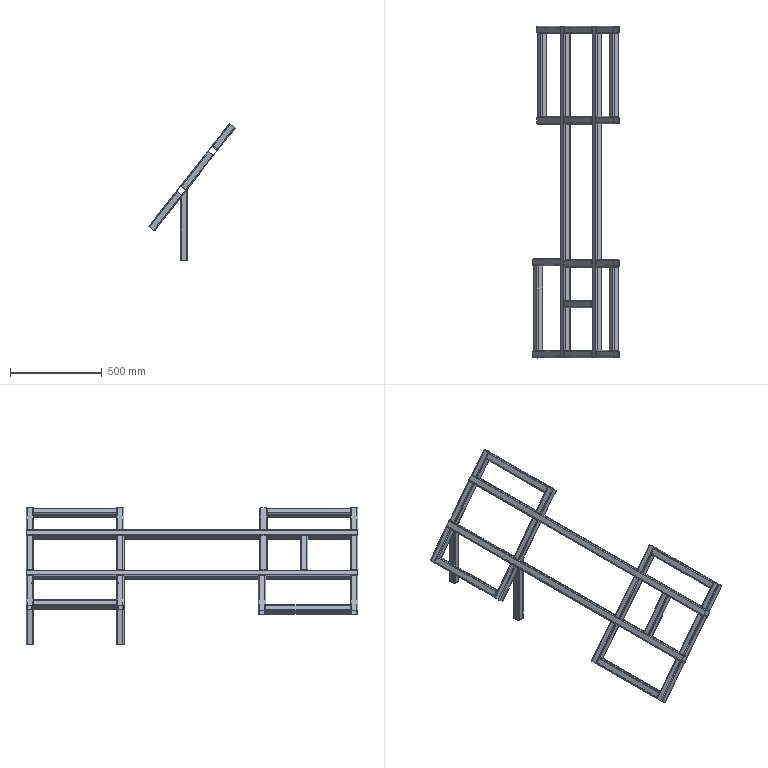Part | STEP file | front baffle frame--20251202 | 21 solids | 378 faces | box 468.919 x 1805 x 743.614 mm | volume 3730425 mm3 | plane 210 | cylinder 168 | commonest cylinder face diameters 12 x92 6 x76